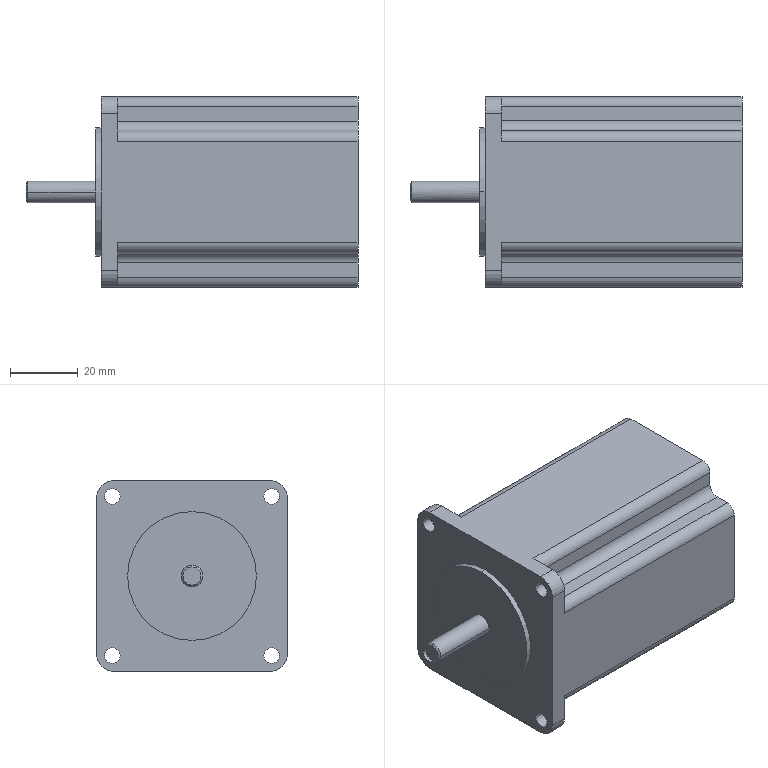Part | STEP file | BS57 Baishan Motor | 1 solid | 50 faces | box 98.2 x 56.4 x 56.4 mm | volume 213692 mm3 | cylinder 28 | plane 20 | cone 2 | commonest cylinder face diameters 6 x12 4.6 x8 10 x4 6.35 x2 38.1 x2